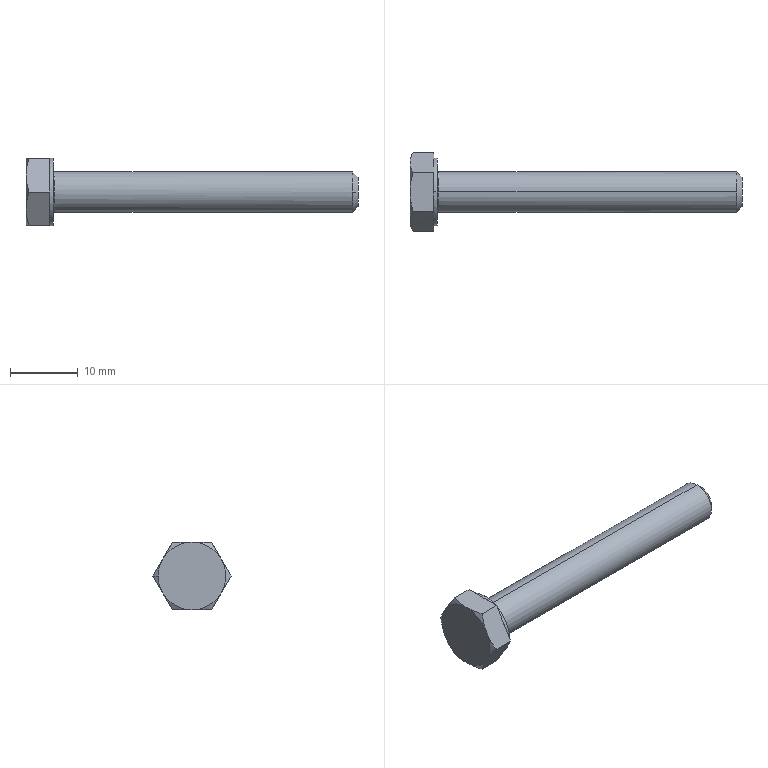Part | STEP file | 1 solid | 30 faces | box 49 x 11.547 x 10.001 mm | volume 1609 mm3 | plane 15 | cone 9 | cylinder 4 | spline 2 | commonest cylinder face diameters 6 x2 10 x2